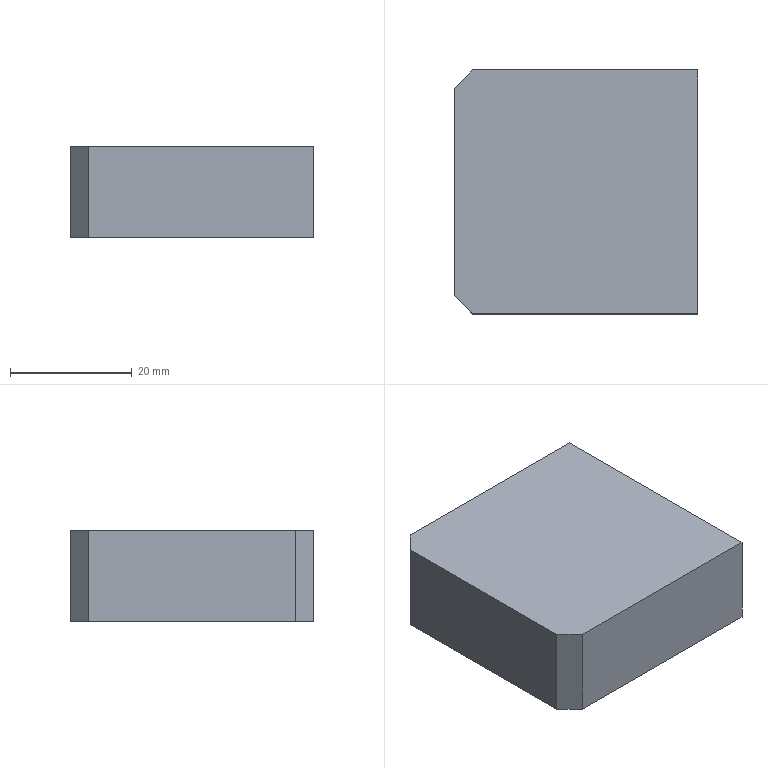Part | NX | 1 solid | 12 faces | box 40 x 40 x 15 mm | volume 23256 mm3 | plane 8 | cone 2 | cylinder 2 | commonest cylinder face diameters 5 x2
STEP:
#1=CARTESIAN_POINT('',(20.,-15.,-2.5));
#2=VERTEX_POINT('',#1);
#3=CARTESIAN_POINT('',(20.,-15.,0.));
#4=DIRECTION('',(1.,0.,0.));
#5=DIRECTION('',(0.,0.,-1.));
#6=AXIS2_PLACEMENT_3D('',#3,#4,#5);
#7=CIRCLE('',#6,2.5);
#8=EDGE_CURVE('',#2,#2,#7,.T.);
#9=ORIENTED_EDGE('',*,*,#8,.F.);
#10=EDGE_LOOP('',(#9));
#11=FACE_BOUND('',#10,.T.);
#12=CARTESIAN_POINT('',(20.,15.,-2.5));
#13=VERTEX_POINT('',#12);
#14=CARTESIAN_POINT('',(20.,15.,0.));
#15=DIRECTION('',(1.,0.,0.));
#16=DIRECTION('',(0.,0.,-1.));
#17=AXIS2_PLACEMENT_3D('',#14,#15,#16);
#18=CIRCLE('',#17,2.5);
#19=EDGE_CURVE('',#13,#13,#18,.T.);
#20=ORIENTED_EDGE('',*,*,#19,.F.);
#21=EDGE_LOOP('',(#20));
#22=FACE_BOUND('',#21,.T.);
#23=CARTESIAN_POINT('',(20.,-20.,-7.5));
#24=VERTEX_POINT('',#23);
#25=CARTESIAN_POINT('',(20.,20.,-7.5));
#26=VERTEX_POINT('',#25);
#27=CARTESIAN_POINT('',(20.,20.,-7.5));
#28=DIRECTION('',(0.,1.,0.));
#29=VECTOR('',#28,1000.);
#30=LINE('',#27,#29);
#31=EDGE_CURVE('',#24,#26,#30,.T.);
#32=ORIENTED_EDGE('',*,*,#31,.T.);
#33=CARTESIAN_POINT('',(20.,20.,7.5));
#34=VERTEX_POINT('',#33);
#35=CARTESIAN_POINT('',(20.,20.,7.5));
#36=DIRECTION('',(0.,0.,-1.));
#37=VECTOR('',#36,1000.);
#38=LINE('',#35,#37);
#39=EDGE_CURVE('',#34,#26,#38,.T.);
#40=ORIENTED_EDGE('',*,*,#39,.F.);
#41=CARTESIAN_POINT('',(20.,-20.,7.5));
#42=VERTEX_POINT('',#41);
#43=CARTESIAN_POINT('',(20.,20.,7.5));
#44=DIRECTION('',(0.,1.,0.));
#45=VECTOR('',#44,1000.);
#46=LINE('',#43,#45);
#47=EDGE_CURVE('',#42,#34,#46,.T.);
#48=ORIENTED_EDGE('',*,*,#47,.F.);
#49=CARTESIAN_POINT('',(20.,-20.,7.5));
#50=DIRECTION('',(0.,0.,-1.));
#51=VECTOR('',#50,1000.);
#52=LINE('',#49,#51);
#53=EDGE_CURVE('',#42,#24,#52,.T.);
#54=ORIENTED_EDGE('',*,*,#53,.T.);
#55=EDGE_LOOP('',(#32,#40,#48,#54));
#56=FACE_BOUND('',#55,.T.);
#57=CARTESIAN_POINT('',(20.,20.,7.5));
#58=DIRECTION('',(-1.,0.,0.));
#59=DIRECTION('',(0.,0.,1.));
#60=AXIS2_PLACEMENT_3D('',#57,#58,#59);
#61=PLANE('',#60);
#62=ADVANCED_FACE('',(#11,#22,#56),#61,.F.);
#63=CARTESIAN_POINT('',(-17.,20.,-7.5));
#64=VERTEX_POINT('',#63);
#65=CARTESIAN_POINT('',(-20.,20.,-7.5));
#66=DIRECTION('',(-1.,0.,0.));
#67=VECTOR('',#66,1000.);
#68=LINE('',#65,#67);
#69=EDGE_CURVE('',#26,#64,#68,.T.);
#70=ORIENTED_EDGE('',*,*,#69,.T.);
#71=CARTESIAN_POINT('',(-17.,20.,7.5));
#72=VERTEX_POINT('',#71);
#73=CARTESIAN_POINT('',(-17.,20.,7.5));
#74=DIRECTION('',(0.,0.,1.));
#75=VECTOR('',#74,1000.);
#76=LINE('',#73,#75);
#77=EDGE_CURVE('',#64,#72,#76,.T.);
#78=ORIENTED_EDGE('',*,*,#77,.T.);
#79=CARTESIAN_POINT('',(-20.,20.,7.5));
#80=DIRECTION('',(-1.,0.,0.));
#81=VECTOR('',#80,1000.);
#82=LINE('',#79,#81);
#83=EDGE_CURVE('',#34,#72,#82,.T.);
#84=ORIENTED_EDGE('',*,*,#83,.F.);
#85=ORIENTED_EDGE('',*,*,#39,.T.);
#86=EDGE_LOOP('',(#70,#78,#84,#85));
#87=FACE_BOUND('',#86,.T.);
#88=CARTESIAN_POINT('',(-20.,20.,7.5));
#89=DIRECTION('',(0.,-1.,0.));
#90=DIRECTION('',(0.,0.,-1.));
#91=AXIS2_PLACEMENT_3D('',#88,#89,#90);
#92=PLANE('',#91);
#93=ADVANCED_FACE('',(#87),#92,.F.);
#94=CARTESIAN_POINT('',(-20.,17.,7.5));
#95=VERTEX_POINT('',#94);
#96=CARTESIAN_POINT('',(-20.,-17.,7.5));
#97=VERTEX_POINT('',#96);
#98=CARTESIAN_POINT('',(-20.,20.,7.5));
#99=DIRECTION('',(0.,-1.,0.));
#100=VECTOR('',#99,1000.);
#101=LINE('',#98,#100);
#102=EDGE_CURVE('',#95,#97,#101,.T.);
#103=ORIENTED_EDGE('',*,*,#102,.F.);
#104=CARTESIAN_POINT('',(-20.,17.,-7.5));
#105=VERTEX_POINT('',#104);
#106=CARTESIAN_POINT('',(-20.,17.,7.5));
#107=DIRECTION('',(0.,0.,-1.));
#108=VECTOR('',#107,1000.);
#109=LINE('',#106,#108);
#110=EDGE_CURVE('',#95,#105,#109,.T.);
#111=ORIENTED_EDGE('',*,*,#110,.T.);
#112=CARTESIAN_POINT('',(-20.,-17.,-7.5));
#113=VERTEX_POINT('',#112);
#114=CARTESIAN_POINT('',(-20.,20.,-7.5));
#115=DIRECTION('',(0.,-1.,0.));
#116=VECTOR('',#115,1000.);
#117=LINE('',#114,#116);
#118=EDGE_CURVE('',#105,#113,#117,.T.);
#119=ORIENTED_EDGE('',*,*,#118,.T.);
#120=CARTESIAN_POINT('',(-20.,-17.,7.5));
#121=DIRECTION('',(0.,0.,1.));
#122=VECTOR('',#121,1000.);
#123=LINE('',#120,#122);
#124=EDGE_CURVE('',#113,#97,#123,.T.);
#125=ORIENTED_EDGE('',*,*,#124,.T.);
#126=EDGE_LOOP('',(#103,#111,#119,#125));
#127=FACE_BOUND('',#126,.T.);
#128=CARTESIAN_POINT('',(-20.,20.,7.5));
#129=DIRECTION('',(1.,0.,0.));
#130=DIRECTION('',(0.,1.,0.));
#131=AXIS2_PLACEMENT_3D('',#128,#129,#130);
#132=PLANE('',#131);
#133=ADVANCED_FACE('',(#127),#132,.F.);
#134=CARTESIAN_POINT('',(-17.,-20.,7.5));
#135=VERTEX_POINT('',#134);
#136=CARTESIAN_POINT('',(-20.,-20.,7.5));
#137=DIRECTION('',(1.,0.,0.));
#138=VECTOR('',#137,1000.);
#139=LINE('',#136,#138);
#140=EDGE_CURVE('',#135,#42,#139,.T.);
#141=ORIENTED_EDGE('',*,*,#140,.F.);
#142=CARTESIAN_POINT('',(-17.,-20.,-7.5));
#143=VERTEX_POINT('',#142);
#144=CARTESIAN_POINT('',(-17.,-20.,7.5));
#145=DIRECTION('',(0.,0.,-1.));
#146=VECTOR('',#145,1000.);
#147=LINE('',#144,#146);
#148=EDGE_CURVE('',#135,#143,#147,.T.);
#149=ORIENTED_EDGE('',*,*,#148,.T.);
#150=CARTESIAN_POINT('',(-20.,-20.,-7.5));
#151=DIRECTION('',(1.,0.,0.));
#152=VECTOR('',#151,1000.);
#153=LINE('',#150,#152);
#154=EDGE_CURVE('',#143,#24,#153,.T.);
#155=ORIENTED_EDGE('',*,*,#154,.T.);
#156=ORIENTED_EDGE('',*,*,#53,.F.);
#157=EDGE_LOOP('',(#141,#149,#155,#156));
#158=FACE_BOUND('',#157,.T.);
#159=CARTESIAN_POINT('',(-20.,-20.,7.5));
#160=DIRECTION('',(0.,1.,0.));
#161=DIRECTION('',(0.,0.,1.));
#162=AXIS2_PLACEMENT_3D('',#159,#160,#161);
#163=PLANE('',#162);
#164=ADVANCED_FACE('',(#158),#163,.F.);
#165=ORIENTED_EDGE('',*,*,#83,.T.);
#166=CARTESIAN_POINT('',(-18.5,18.5,7.5));
#167=DIRECTION('',(0.7071,0.7071,0.));
#168=VECTOR('',#167,1000.);
#169=LINE('',#166,#168);
#170=EDGE_CURVE('',#72,#95,#169,.F.);
#171=ORIENTED_EDGE('',*,*,#170,.T.);
#172=ORIENTED_EDGE('',*,*,#102,.T.);
#173=CARTESIAN_POINT('',(-18.5,-18.5,7.5));
#174=DIRECTION('',(-0.7071,0.7071,0.));
#175=VECTOR('',#174,1000.);
#176=LINE('',#173,#175);
#177=EDGE_CURVE('',#97,#135,#176,.F.);
#178=ORIENTED_EDGE('',*,*,#177,.T.);
#179=ORIENTED_EDGE('',*,*,#140,.T.);
#180=ORIENTED_EDGE('',*,*,#47,.T.);
#181=EDGE_LOOP('',(#165,#171,#172,#178,#179,#180));
#182=FACE_BOUND('',#181,.T.);
#183=CARTESIAN_POINT('',(0.,0.,7.5));
#184=DIRECTION('',(0.,0.,1.));
#185=DIRECTION('',(1.,0.,0.));
#186=AXIS2_PLACEMENT_3D('',#183,#184,#185);
#187=PLANE('',#186);
#188=ADVANCED_FACE('',(#182),#187,.T.);
#189=ORIENTED_EDGE('',*,*,#118,.F.);
#190=CARTESIAN_POINT('',(-20.,17.,-7.5));
#191=DIRECTION('',(-0.7071,-0.7071,0.));
#192=VECTOR('',#191,1000.);
#193=LINE('',#190,#192);
#194=EDGE_CURVE('',#105,#64,#193,.F.);
#195=ORIENTED_EDGE('',*,*,#194,.T.);
#196=ORIENTED_EDGE('',*,*,#69,.F.);
#197=ORIENTED_EDGE('',*,*,#31,.F.);
#198=ORIENTED_EDGE('',*,*,#154,.F.);
#199=CARTESIAN_POINT('',(-17.,-20.,-7.5));
#200=DIRECTION('',(0.7071,-0.7071,0.));
#201=VECTOR('',#200,1000.);
#202=LINE('',#199,#201);
#203=EDGE_CURVE('',#143,#113,#202,.F.);
#204=ORIENTED_EDGE('',*,*,#203,.T.);
#205=EDGE_LOOP('',(#189,#195,#196,#197,#198,#204));
#206=FACE_BOUND('',#205,.T.);
#207=CARTESIAN_POINT('',(0.,0.,-7.5));
#208=DIRECTION('',(0.,0.,1.));
#209=DIRECTION('',(1.,0.,0.));
#210=AXIS2_PLACEMENT_3D('',#207,#208,#209);
#211=PLANE('',#210);
#212=ADVANCED_FACE('',(#206),#211,.F.);
#213=CARTESIAN_POINT('',(3.498,15.,0.));
#214=VERTEX_POINT('',#213);
#215=VERTEX_LOOP('',#214);
#216=FACE_BOUND('',#215,.T.);
#217=CARTESIAN_POINT('',(5.,15.,-2.5));
#218=VERTEX_POINT('',#217);
#219=CARTESIAN_POINT('',(5.,15.,0.));
#220=DIRECTION('',(1.,0.,0.));
#221=DIRECTION('',(0.,0.,-1.));
#222=AXIS2_PLACEMENT_3D('',#219,#220,#221);
#223=CIRCLE('',#222,2.5);
#224=EDGE_CURVE('',#218,#218,#223,.T.);
#225=ORIENTED_EDGE('',*,*,#224,.T.);
#226=EDGE_LOOP('',(#225));
#227=FACE_BOUND('',#226,.T.);
#228=CARTESIAN_POINT('',(5.,15.,0.));
#229=DIRECTION('',(1.,0.,0.));
#230=DIRECTION('',(0.,0.,-1.));
#231=AXIS2_PLACEMENT_3D('',#228,#229,#230);
#232=CONICAL_SURFACE('',#231,2.5,1.03);
#233=ADVANCED_FACE('',(#216,#227),#232,.F.);
#234=ORIENTED_EDGE('',*,*,#224,.F.);
#235=EDGE_LOOP('',(#234));
#236=FACE_BOUND('',#235,.T.);
#237=ORIENTED_EDGE('',*,*,#19,.T.);
#238=EDGE_LOOP('',(#237));
#239=FACE_BOUND('',#238,.T.);
#240=CARTESIAN_POINT('',(20.,15.,0.));
#241=DIRECTION('',(1.,0.,0.));
#242=DIRECTION('',(0.,0.,-1.));
#243=AXIS2_PLACEMENT_3D('',#240,#241,#242);
#244=CYLINDRICAL_SURFACE('',#243,2.5);
#245=ADVANCED_FACE('',(#236,#239),#244,.F.);
#246=CARTESIAN_POINT('',(3.498,-15.,0.));
#247=VERTEX_POINT('',#246);
#248=VERTEX_LOOP('',#247);
#249=FACE_BOUND('',#248,.T.);
#250=CARTESIAN_POINT('',(5.,-15.,-2.5));
#251=VERTEX_POINT('',#250);
#252=CARTESIAN_POINT('',(5.,-15.,0.));
#253=DIRECTION('',(1.,0.,0.));
#254=DIRECTION('',(0.,0.,-1.));
#255=AXIS2_PLACEMENT_3D('',#252,#253,#254);
#256=CIRCLE('',#255,2.5);
#257=EDGE_CURVE('',#251,#251,#256,.T.);
#258=ORIENTED_EDGE('',*,*,#257,.T.);
#259=EDGE_LOOP('',(#258));
#260=FACE_BOUND('',#259,.T.);
#261=CARTESIAN_POINT('',(5.,-15.,0.));
#262=DIRECTION('',(1.,0.,0.));
#263=DIRECTION('',(0.,0.,-1.));
#264=AXIS2_PLACEMENT_3D('',#261,#262,#263);
#265=CONICAL_SURFACE('',#264,2.5,1.03);
#266=ADVANCED_FACE('',(#249,#260),#265,.F.);
#267=ORIENTED_EDGE('',*,*,#257,.F.);
#268=EDGE_LOOP('',(#267));
#269=FACE_BOUND('',#268,.T.);
#270=ORIENTED_EDGE('',*,*,#8,.T.);
#271=EDGE_LOOP('',(#270));
#272=FACE_BOUND('',#271,.T.);
#273=CARTESIAN_POINT('',(20.,-15.,0.));
#274=DIRECTION('',(1.,0.,0.));
#275=DIRECTION('',(0.,0.,-1.));
#276=AXIS2_PLACEMENT_3D('',#273,#274,#275);
#277=CYLINDRICAL_SURFACE('',#276,2.5);
#278=ADVANCED_FACE('',(#269,#272),#277,.F.);
#279=ORIENTED_EDGE('',*,*,#170,.F.);
#280=ORIENTED_EDGE('',*,*,#77,.F.);
#281=ORIENTED_EDGE('',*,*,#194,.F.);
#282=ORIENTED_EDGE('',*,*,#110,.F.);
#283=EDGE_LOOP('',(#279,#280,#281,#282));
#284=FACE_BOUND('',#283,.T.);
#285=CARTESIAN_POINT('',(-20.,17.,7.5));
#286=DIRECTION('',(0.7071,-0.7071,0.));
#287=DIRECTION('',(0.,0.,-1.));
#288=AXIS2_PLACEMENT_3D('',#285,#286,#287);
#289=PLANE('',#288);
#290=ADVANCED_FACE('',(#284),#289,.F.);
#291=ORIENTED_EDGE('',*,*,#177,.F.);
#292=ORIENTED_EDGE('',*,*,#124,.F.);
#293=ORIENTED_EDGE('',*,*,#203,.F.);
#294=ORIENTED_EDGE('',*,*,#148,.F.);
#295=EDGE_LOOP('',(#291,#292,#293,#294));
#296=FACE_BOUND('',#295,.T.);
#297=CARTESIAN_POINT('',(-17.,-20.,7.5));
#298=DIRECTION('',(0.7071,0.7071,0.));
#299=DIRECTION('',(0.,0.,-1.));
#300=AXIS2_PLACEMENT_3D('',#297,#298,#299);
#301=PLANE('',#300);
#302=ADVANCED_FACE('',(#296),#301,.F.);
#303=CLOSED_SHELL('',(#62,#93,#133,#164,#188,#212,#233,#245,#266,#278,#290,#302));
#304=MANIFOLD_SOLID_BREP('',#303);
#305=(LENGTH_UNIT()NAMED_UNIT(*)SI_UNIT(.MILLI.,.METRE.));
#306=UNCERTAINTY_MEASURE_WITH_UNIT(LENGTH_MEASURE(0.00001),#305,'','');
#307=(NAMED_UNIT(*)PLANE_ANGLE_UNIT()SI_UNIT($,.RADIAN.));
#308=(NAMED_UNIT(*)SI_UNIT($,.STERADIAN.)SOLID_ANGLE_UNIT());
#309=(GEOMETRIC_REPRESENTATION_CONTEXT(3)GLOBAL_UNCERTAINTY_ASSIGNED_CONTEXT((#306))GLOBAL_UNIT_ASSIGNED_CONTEXT((#305,#307,#308))REPRESENTATION_CONTEXT('',''));
#310=ADVANCED_BREP_SHAPE_REPRESENTATION('',(#304),#309);